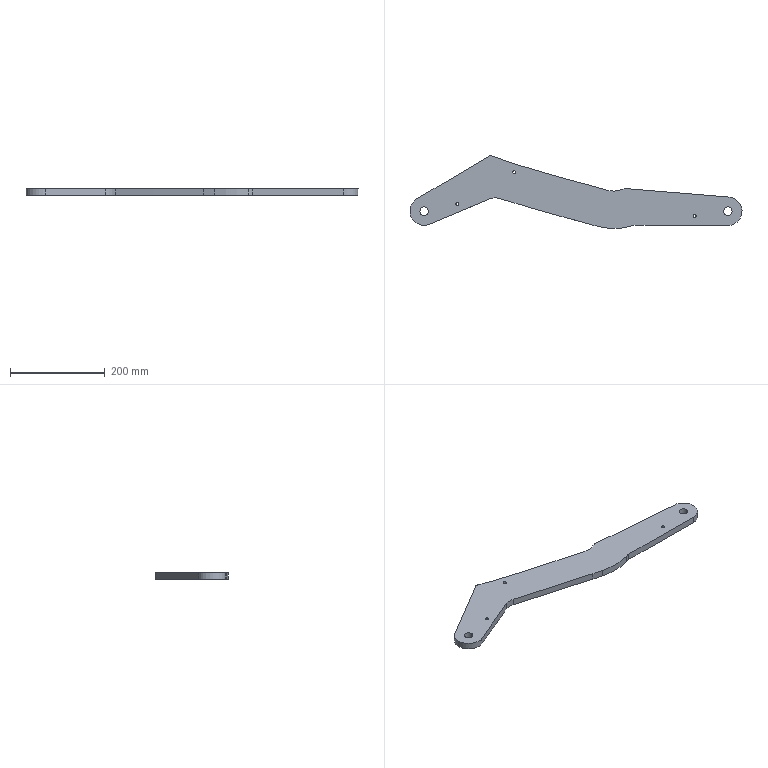NC program | NX | posted with a generic post | part box 700 x 153.975 x 14 mm
Lines 4525 to 6173 of 6173, first 1547 of 1637 lines:
(SPOT_FACING_COPY , TOOL : D12)
N9042 M6
N9044 G54
N9046 G17 G0 G90 X640. Y0. S0 M3
N9048 G43 Z117. H0
N9050 G94 G82 G99 Z17. F250. P200 R23.
N9052 X0.
N9054 G80
N9056 G0 X0. Y0. Z117.
N9058 M5
(ZLEVEL_PROFILE , TOOL : D20R0)
N9060 M6
N9062 G54
N9064 G17 G0 G90 X590.572 Y-39.778 S4500 M3
N9066 G43 Z117. H0
N9068 Z15.
N9070 G94 G1 X639.806 Y-40. Z14.141 F3000.
N9072 X641.356 Y-40.007 Z14.114
N9074 X645.633 Y-39.632 Z14.039
N9076 X649.845 Y-38.8 Z13.964
N9078 X653.944 Y-37.523 Z13.889
N9080 X657.883 Y-35.814 Z13.814
N9082 X661.616 Y-33.692 Z13.739
N9084 X665.1 Y-31.183 Z13.664
N9086 X668.295 Y-28.316 Z13.589
N9088 X671.165 Y-25.122 Z13.514
N9090 X673.677 Y-21.64 Z13.439
N9092 X675.25 Y-18.97 Z13.385
N9094 X677.089 Y-15.059 Z13.31
N9096 X678.497 Y-10.973 Z13.234
N9098 X679.455 Y-6.758 Z13.159
N9100 X679.954 Y-2.465 Z13.083
N9102 X679.987 Y1.857 Z13.008
N9104 X679.554 Y6.157 Z12.932
N9106 X678.659 Y10.385 Z12.857
N9108 X677.314 Y14.493 Z12.781
N9110 X675.534 Y18.431 Z12.706
N9112 X673.34 Y22.155 Z12.631
N9114 X670.757 Y25.62 Z12.555
N9116 X667.816 Y28.787 Z12.48
N9118 X664.55 Y31.618 Z12.404
N9120 X660.998 Y34.08 Z12.329
N9122 X657.202 Y36.146 Z12.253
N9124 X653.205 Y37.789 Z12.178
N9126 X649.053 Y38.993 Z12.102
N9128 X644.797 Y39.742 Z12.027
N9130 X643.252 Y39.868 Z12.
N9132 G2 X639.806 Y-40. R40.
N9134 G1 X448.418 Y-39.138
N9136 G3 X442.249 Y-40.086 R20.
N9138 G2 X365.067 Y-42.198 R139.056
N9140 X207.429 Y1.588 R6700.642
N9142 X163.525 Y14.814 R2452.181
N9144 G1 X156.009 Y17.183
N9146 G3 X142.137 Y16.562 R20.
N9148 G1 X15.549 Y-36.854
N9150 G2 X-20.445 Y34.38 R40.
N9152 G1 Z10.
N9154 G3 X15.549 Y-36.854 R40.
N9156 G1 X142.137 Y16.562
N9158 G2 X156.009 Y17.183 R20.
N9160 G3 X205.106 Y2.266 R2244.387
N9162 X365.066 Y-42.198 R6672.834
N9164 X442.249 Y-40.086 R138.995
N9166 G2 X448.418 Y-39.138 R20.
N9168 G1 X639.806 Y-40.
N9170 G3 X643.252 Y39.868 R40.
N9172 G1 Z8.
N9174 G2 X639.806 Y-40. R40.
N9176 G1 X448.418 Y-39.138
N9178 G3 X442.249 Y-40.086 R20.
N9180 G2 X365.065 Y-42.198 R138.996
N9182 X205.106 Y2.265 R6680.91
N9184 X156.009 Y17.183 R2242.923
N9186 G3 X142.137 Y16.562 R20.
N9188 G1 X15.549 Y-36.854
N9190 G2 X-20.445 Y34.38 R40.
N9192 G1 Z6.
N9194 G3 X15.549 Y-36.854 R40.
N9196 G1 X142.137 Y16.562
N9198 G2 X156.009 Y17.183 R20.
N9200 G3 X205.106 Y2.265 R2241.461
N9202 X364.863 Y-42.146 R6694.497
N9204 X442.249 Y-40.086 R139.003
N9206 G2 X448.418 Y-39.138 R20.
N9208 G1 X639.806 Y-40.
N9210 G3 X643.252 Y39.868 R40.
N9212 G1 Z4.
N9214 G2 X639.806 Y-40. R40.
N9216 G1 X448.418 Y-39.138
N9218 G3 X442.249 Y-40.086 R20.
N9220 G2 X364.863 Y-42.147 R138.995
N9222 X205.106 Y2.264 R6704.295
N9224 X156.009 Y17.183 R2239.999
N9226 G3 X142.137 Y16.562 R20.
N9228 G1 X15.549 Y-36.854
N9230 G2 X-20.445 Y34.38 R40.
N9232 G1 Z2.
N9234 G3 X15.549 Y-36.854 R40.
N9236 G1 X142.137 Y16.562
N9238 G2 X156.009 Y17.183 R20.
N9240 G3 X205.106 Y2.264 R2242.559
N9242 X364.863 Y-42.148 R6672.146
N9244 X442.249 Y-40.086 R138.997
N9246 G2 X448.418 Y-39.138 R20.
N9248 G1 X639.806 Y-40.
N9250 G3 X643.252 Y39.868 R40.
N9252 G1 Z0.
N9254 G2 X639.806 Y-40. R40.
N9256 G1 X448.418 Y-39.138
N9258 G3 X442.249 Y-40.086 R20.
N9260 G2 X364.863 Y-42.148 R138.999
N9262 X205.106 Y2.263 R6621.095
N9264 X156.009 Y17.183 R2197.08
N9266 G3 X142.137 Y16.562 R20.
N9268 G1 X15.549 Y-36.854
N9270 G2 X-20.445 Y34.38 R40.
N9272 G1 Z3.
N9274 G0 Z117.
N9276 M5
(CONTOUR_TEXT , TOOL : D0.1)
N9278 M6
N9280 G54
N9282 G17 G0 G90 X143.989 Y116.042 S2000 M3
N9284 G43 Z117. H0
N9286 Z17.01
N9288 G94 G1 Z14. F1000.
N9290 X140.878 Y26.737
N9292 Z17.01
N9294 G0 Z117.
N9296 X340. Y56.736
N9298 Z17.01
N9300 G1 Z14.
N9302 Y56.686
N9304 Y-25.158
N9306 Z17.01
N9308 G0 Z117.
N9310 X365. Y49.967
N9312 Z17.01
N9314 G1 Z14.
N9316 Y49.902
N9318 Y-31.828
N9320 Y-31.838
N9322 Z17.01
N9324 G0 Z117.
N9326 M5
(SPOT_FACING , TOOL : D18)
N9328 M6
N9330 G54
N9332 G17 G0 G90 X640. Y0. S0 M3
N9334 G43 Z117. H0
N9336 G94 G82 G99 Z14. F250. P200 R20.
N9338 X0.
N9340 G80
N9342 G0 X0. Y0. Z117.
N9344 M5
(SPOT_FACING_1 , TOOL : D6.35)
N9346 M6
N9348 G54
N9350 G17 G0 G90 X570. Y-10. S0 M3
N9352 G43 Z117. H0
N9354 G94 G82 G99 Z14. F250. P200 R20.
N9356 X190. Y82.
N9358 X70. Y15.
N9360 G80
N9362 G0 X70. Y15. Z117.
N9364 M5
(ZLEVEL_PROFILE_COPY_COPY , TOOL : D16R3)
N9366 M6
N9368 G54
N9370 G17 G0 G90 X-407.756 Y50.913 S4500 M3
N9372 G43 Z100. H0
N9374 Z3.015
N9376 G94 G1 Z0.015 F3000.
N9378 G3 X-401.133 Y50.207 R42.151
N9380 G1 Z3.015
N9382 G0 Z100.
N9384 X-387.654 Y52.009
N9386 Z3.015
N9388 G1 Z0.015
N9390 G3 X-383.592 Y53.088 R6599.663
N9392 G1 Z3.015
N9394 G0 Z100.
N9396 X-378.518 Y54.438
N9398 Z3.015
N9400 G1 Z0.015
N9402 G3 X-373.217 Y55.854 R6599.663
N9404 G1 Z3.015
N9406 G0 Z100.
N9408 X-369.755 Y56.781
N9410 Z3.015
N9412 G1 Z0.015
N9414 G3 X-366.871 Y57.555 R6599.663
N9416 G1 Z3.015
N9418 G0 Z100.
N9420 X-358.003 Y59.944
N9422 Z3.015
N9424 G1 Z0.015
N9426 G3 X-352.957 Y61.309 R6599.663
N9428 G1 Z3.015
N9430 G0 Z100.
N9432 X-330.802 Y67.353
N9434 Z3.015
N9436 G1 Z0.015
N9438 G3 X-327.793 Y68.181 R6599.663
N9440 G1 Z3.015
N9442 G0 Z100.
N9444 X-298.143 Y76.415
N9446 Z3.015
N9448 G1 Z0.015
N9450 G3 X-296.135 Y76.978 R6599.663
N9452 G1 Z3.015
N9454 G0 Z100.
N9456 X-290.769 Y78.486
N9458 Z3.015
N9460 G1 Z0.015
N9462 G3 X-288.272 Y79.189 R6599.663
N9464 G1 Z3.015
N9466 G0 Z100.
N9468 X-248.142 Y90.638
N9470 Z3.015
N9472 G1 Z0.015
N9474 G3 X-246.973 Y90.976 R6599.663
N9476 G1 Z3.015
N9478 G0 Z100.
N9480 X-211.221 Y101.494
N9482 Z3.015
N9484 G1 Z0.015
N9486 G3 X-207.58 Y102.599 R2171.481
N9488 G1 Z3.015
N9490 G0 Z100.
N9492 X-153.644 Y120.541
N9494 Z3.015
N9496 G1 Z0.015
N9498 G3 X-150.685 Y121.74 R241.278
N9500 G1 Z3.015
N9502 G0 Z100.
N9504 X-147.619 Y123.03
N9506 Z3.015
N9508 G1 Z0.015
N9510 G3 X-145.285 Y124.045 R241.278
N9512 G2 X-141.102 Y125.139 R12.975
N9514 G1 Z3.015
N9516 G0 Z100.
N9518 X-415.341 Y53.085
N9520 Z3.015
N9522 G1 Z0.015
N9524 G3 X-411.202 Y51.709 R42.151
N9526 G1 Z3.015
N9528 G0 Z100.
N9530 X-125.772 Y118.879
N9532 Z2.866
N9534 G1 X19.35 Y32.635 Z-0.081
N9536 X21.902 Y31.119 Z-0.133
N9538 X21.939 Y31.096 Z-0.134
N9540 X21.976 Y31.074
N9542 X21.902 Y31.119
N9544 X19.35 Y32.635
N9546 X-133.408 Y123.417
N9548 G3 X-145.285 Y124.046 R12.983
N9550 G2 X-161.394 Y117.61 R244.177
N9552 X-192.374 Y107.278 R743.347
N9554 X-243.617 Y91.937 R2595.945
N9556 X-389.036 Y51.644 R6726.527
N9558 X-418.12 Y54.295 R42.063
N9560 G3 X-424.947 Y55.612 R13.128
N9562 G1 X-643.044 Y37.818
N9564 X-645.25 Y37.626
N9566 Z-0.284
N9568 X-643.044 Y37.818
N9570 X-424.947 Y55.612
N9572 G2 X-418.12 Y54.295 R13.112
N9574 G3 X-389.036 Y51.645 R42.063
N9576 X-243.617 Y91.938 R6726.001
N9578 X-192.374 Y107.278 R2596.179
N9580 X-161.396 Y117.61 R743.332
N9582 X-145.285 Y124.047 R244.134
N9584 G2 X-133.408 Y123.417 R12.974
N9586 G1 X19.35 Y32.635
N9588 X21.902 Y31.119
N9590 X21.976 Y31.074
N9592 Z-0.433
N9594 X21.902 Y31.119
N9596 X19.35 Y32.635
N9598 X-133.408 Y123.417
N9600 G3 X-145.285 Y124.048 R12.971
N9602 G2 X-161.398 Y117.61 R244.08
N9604 X-192.374 Y107.279 R743.308
N9606 X-243.617 Y91.938 R2596.414
N9608 X-389.036 Y51.645 R6725.354
N9610 X-418.12 Y54.296 R42.063
N9612 G3 X-424.947 Y55.612 R13.096
N9614 G1 X-643.044 Y37.818
N9616 X-645.25 Y37.626
N9618 Z-0.582
N9620 X-643.044 Y37.818
N9622 X-424.947 Y55.612
N9624 G2 X-418.12 Y54.297 R13.085
N9626 G3 X-389.036 Y51.646 R42.063
N9628 X-243.617 Y91.939 R6724.841
N9630 X-192.374 Y107.28 R2596.46
N9632 X-161.4 Y117.61 R743.27
N9634 X-145.285 Y124.049 R244.026
N9636 G2 X-133.408 Y123.417 R12.969
N9638 G1 X19.35 Y32.635
N9640 X21.902 Y31.119
N9642 X21.976 Y31.074
N9644 Z-0.731
N9646 X21.902 Y31.119
N9648 X19.35 Y32.635
N9650 X-133.408 Y123.417
N9652 G3 X-145.285 Y124.05 R12.969
N9654 G2 X-161.402 Y117.61 R243.973
N9656 X-192.374 Y107.28 R743.229
N9658 X-243.617 Y91.94 R2596.058
N9660 X-389.036 Y51.647 R6724.335
N9662 X-418.12 Y54.298 R42.063
N9664 G3 X-424.947 Y55.612 R13.081
N9666 G1 X-643.044 Y37.818
N9668 X-645.25 Y37.626
N9670 Z-0.881
N9672 X-643.044 Y37.818
N9674 X-424.947 Y55.612
N9676 G2 X-418.12 Y54.299 R13.079
N9678 G3 X-389.036 Y51.648 R42.062
N9680 X-243.617 Y91.94 R6723.829
N9682 X-192.374 Y107.281 R2595.627
N9684 X-161.404 Y117.61 R743.186
N9686 X-145.285 Y124.05 R243.919
N9688 G2 X-133.408 Y123.417 R12.969
N9690 G1 X19.35 Y32.635
N9692 X21.902 Y31.119
N9694 X21.976 Y31.074
N9696 Z-1.03
N9698 X21.902 Y31.119
N9700 X19.35 Y32.635
N9702 X-133.408 Y123.417
N9704 G3 X-145.285 Y124.051 R12.968
N9706 G2 X-161.406 Y117.61 R243.88
N9708 X-192.374 Y107.282 R743.005
N9710 X-243.617 Y91.941 R2595.195
N9712 X-389.036 Y51.648 R6723.968
N9714 X-418.12 Y54.299 R42.063
N9716 G3 X-424.947 Y55.612 R13.077
N9718 G1 X-643.044 Y37.818
N9720 X-645.25 Y37.626
N9722 X-645.251 Y37.638 Z-1.179
N9724 X-643.044 Y37.818
N9726 X-424.947 Y55.612
N9728 G2 X-418.12 Y54.3 R13.075
N9730 G3 X-389.036 Y51.649 R42.063
N9732 X-243.617 Y91.942 R6724.339
N9734 X-192.374 Y107.282 R2594.764
N9736 X-161.408 Y117.61 R743.099
N9738 X-145.285 Y124.052 R243.869
N9740 G2 X-133.408 Y123.417 R12.968
N9742 G1 X19.35 Y32.635
N9744 X21.902 Y31.119
N9746 X21.976 Y31.074
N9748 Z-1.328
N9750 X19.35 Y32.635
N9752 X-133.408 Y123.417
N9754 G3 X-145.285 Y124.053 R12.968
N9756 G2 X-161.409 Y117.61 R243.819
N9758 X-192.374 Y107.283 R743.193
N9760 X-243.617 Y91.942 R2594.333
N9762 X-389.036 Y51.65 R6724.711
N9764 X-418.12 Y54.301 R42.062
N9766 G3 X-424.947 Y55.612 R13.073
N9768 G1 X-643.044 Y37.818
N9770 X-645.251 Y37.638
N9772 Z-1.478
N9774 X-643.044 Y37.818
N9776 X-424.947 Y55.612
N9778 G2 X-418.12 Y54.302 R13.071
N9780 G3 X-389.036 Y51.651 R42.061
N9782 X-243.617 Y91.943 R6725.083
N9784 X-192.374 Y107.284 R2593.902
N9786 X-161.411 Y117.61 R743.288
N9788 X-145.285 Y124.054 R243.688
N9790 G2 X-133.408 Y123.417 R12.968
N9792 G1 X19.35 Y32.635
N9794 X21.902 Y31.119
N9796 X21.976 Y31.074
N9798 Z-1.627
N9800 X21.902 Y31.119
N9802 X19.35 Y32.635
N9804 X-133.408 Y123.417
N9806 G3 X-145.285 Y124.055 R12.968
N9808 G2 X-161.413 Y117.61 R243.517
N9810 X-192.374 Y107.284 R743.382
N9812 X-243.617 Y91.944 R2593.471
N9814 X-389.036 Y51.651 R6725.454
N9816 X-418.12 Y54.303 R42.06
N9818 G3 X-424.947 Y55.612 R13.069
N9820 G1 X-643.044 Y37.818
N9822 X-645.25 Y37.626
N9824 Z-1.776
N9826 X-643.044 Y37.818
N9828 X-424.947 Y55.612
N9830 G2 X-418.12 Y54.303 R13.068
N9832 G3 X-389.036 Y51.652 R42.059
N9834 X-243.617 Y91.944 R6725.826
N9836 X-193.759 Y106.853 R2626.625
N9838 X-163.29 Y116.934 R784.546
N9840 X-145.285 Y124.056 R254.256
N9842 G2 X-133.408 Y123.417 R12.97
N9844 G1 X19.35 Y32.635
N9846 X21.976 Y31.074
N9848 Z-1.925
N9850 X19.35 Y32.635
N9852 X-133.408 Y123.417
N9854 G3 X-145.285 Y124.057 R12.971
N9856 G2 X-163.29 Y116.935 R253.869
N9858 X-193.759 Y106.853 R784.382
N9860 X-243.617 Y91.945 R2625.972
N9862 X-389.036 Y51.653 R6726.197
N9864 X-418.12 Y54.304 R42.058
N9866 G3 X-424.947 Y55.612 R13.067
N9868 G1 X-643.044 Y37.818
N9870 X-645.25 Y37.626
N9872 Z-2.075
N9874 X-643.044 Y37.818
N9876 X-424.947 Y55.612
N9878 G2 X-418.12 Y54.305 R13.066
N9880 G3 X-389.036 Y51.653 R42.057
N9882 X-243.617 Y91.945 R6727.425
N9884 X-192.374 Y107.286 R2594.029
N9886 X-161.418 Y117.61 R742.762
N9888 X-145.285 Y124.058 R242.584
N9890 G2 X-133.408 Y123.417 R12.972
N9892 G1 X19.35 Y32.635
N9894 X21.976 Y31.074
N9896 Z-2.224
N9898 X19.35 Y32.635
N9900 X-133.408 Y123.417
N9902 G3 X-145.285 Y124.059 R12.974
N9904 G2 X-161.42 Y117.61 R242.183
N9906 X-192.374 Y107.286 R741.914
N9908 X-243.617 Y91.946 R2595.715
N9910 X-389.036 Y51.654 R6732.513
N9912 X-418.12 Y54.306 R42.055
N9914 G3 X-424.947 Y55.612 R13.067
N9916 G1 X-643.044 Y37.818
N9918 X-645.25 Y37.626
N9920 Z-2.373
N9922 X-643.044 Y37.818
N9924 X-424.947 Y55.612
N9926 G2 X-418.12 Y54.306 R13.072
N9928 G3 X-389.036 Y51.654 R42.054
N9930 X-232.193 Y95.277 R6557.333
N9932 X-186.834 Y109.038 R2105.117
N9934 X-161.422 Y117.61 R671.478
N9936 X-145.285 Y124.06 R241.607
N9938 G2 X-133.408 Y123.417 R12.976
N9940 G1 X19.35 Y32.635
N9942 X21.976 Y31.074
N9944 Z-2.522
N9946 X19.35 Y32.635
N9948 X-133.408 Y123.417
N9950 G3 X-145.285 Y124.061 R12.976
N9952 G2 X-161.423 Y117.61 R241.158
N9954 X-186.834 Y109.038 R670.893
N9956 X-233.922 Y94.773 R2161.711
N9958 X-389.036 Y51.655 R6568.584
N9960 X-418.12 Y54.307 R42.052
N9962 G3 X-424.947 Y55.612 R13.079
N9964 G1 X-643.044 Y37.818
N9966 X-645.25 Y37.626
N9968 Z-2.672
N9970 X-643.044 Y37.818
N9972 X-424.947 Y55.612
N9974 G2 X-418.12 Y54.308 R13.085
N9976 G3 X-389.036 Y51.655 R42.05
N9978 X-235.307 Y94.369 R6591.52
N9980 X-189.604 Y108.163 R2253.663
N9982 X-161.425 Y117.61 R696.975
N9984 X-145.285 Y124.062 R240.518
N9986 G2 X-133.408 Y123.417 R12.977
N9988 G1 X19.35 Y32.635
N9990 X21.976 Y31.074
N9992 Z-2.821
N9994 X19.35 Y32.635
N9996 X-133.408 Y123.417
N9998 G3 X-145.285 Y124.063 R12.978
N10000 G2 X-161.427 Y117.61 R243.838
N10002 X-189.604 Y108.163 R697.021
N10004 X-232.583 Y95.164 R2231.213
N10006 X-389.036 Y51.656 R6582.428
N10008 X-418.12 Y54.309 R42.048
N10010 G3 X-424.947 Y55.612 R13.091
N10012 G1 X-643.044 Y37.818
N10014 X-645.25 Y37.626
N10016 Z-2.97
N10018 X-643.044 Y37.818
N10020 X-424.947 Y55.612
N10022 G2 X-418.12 Y54.31 R13.097
N10024 G3 X-389.036 Y51.656 R42.046
N10026 X-235.307 Y94.37 R6605.781
N10028 X-186.834 Y109.04 R2185.124
N10030 X-161.429 Y117.61 R678.962
N10032 X-145.285 Y124.064 R243.704
N10034 G2 X-133.408 Y123.417 R12.98
N10036 G1 X19.35 Y32.635
N10038 X21.976 Y31.074
N10040 Z-3.119
N10042 X19.383 Y32.615
N10044 X-133.408 Y123.417
N10046 G3 X-145.285 Y124.065 R12.956
N10048 G2 X-160.135 Y118.088 R230.666
N10050 X-186.834 Y109.042 R650.105
N10052 X-232.454 Y95.204 R2166.728
N10054 X-388.833 Y51.712 R6643.891
N10056 X-418.12 Y54.311 R42.064
N10058 G3 X-424.925 Y55.614 R12.998
N10060 G1 X-643.085 Y37.814
N10062 X-645.25 Y37.626
N10064 Z-3.269
N10066 X-643.085 Y37.814
N10068 X-424.923 Y55.614
N10070 G2 X-418.12 Y54.311 R13.
N10072 G3 X-388.836 Y51.712 R42.063
N10074 X-232.454 Y95.205 R6643.863
N10076 X-186.834 Y109.043 R2167.21
N10078 X-160.135 Y118.088 R649.315
N10080 X-145.285 Y124.066 R230.896
N10082 G2 X-133.408 Y123.417 R12.956
N10084 G1 X19.383 Y32.615
N10086 X21.976 Y31.074
N10088 Z-3.418
N10090 X19.383 Y32.615
N10092 X-133.408 Y123.417
N10094 G3 X-145.285 Y124.067 R12.956
N10096 G2 X-160.135 Y118.089 R230.903
N10098 X-186.834 Y109.043 R646.14
N10100 X-232.455 Y95.206 R2167.693
N10102 X-388.839 Y51.712 R6643.82
N10104 X-418.12 Y54.312 R42.062
N10106 G3 X-424.922 Y55.614 R13.002
N10108 G1 X-643.085 Y37.814
N10110 X-645.25 Y37.626
N10112 Z-3.567
N10114 X-643.085 Y37.814
N10116 X-424.92 Y55.614
N10118 G2 X-418.12 Y54.313 R13.004
N10120 G3 X-388.842 Y51.712 R42.061
N10122 X-232.455 Y95.206 R6643.759
N10124 X-186.834 Y109.044 R2168.176
N10126 X-160.136 Y118.09 R659.938
N10128 X-145.285 Y124.068 R230.911
N10130 G2 X-133.408 Y123.417 R12.957
N10132 G1 X19.383 Y32.615
N10134 X21.976 Y31.074
N10136 Z-3.716
N10138 X19.383 Y32.615
N10140 X-133.408 Y123.417
N10142 G3 X-145.285 Y124.069 R12.957
N10144 G2 X-160.136 Y118.09 R230.918
N10146 X-186.834 Y109.044 R659.332
N10148 X-232.455 Y95.207 R2168.659
N10150 X-389.036 Y51.662 R6578.665
N10152 X-418.12 Y54.314 R42.043
N10154 G3 X-424.919 Y55.614 R13.006
N10156 G1 X-643.085 Y37.814
N10158 X-645.25 Y37.626
N10160 Z-3.866
N10162 X-643.085 Y37.814
N10164 X-424.917 Y55.614
N10166 G2 X-418.12 Y54.315 R13.009
N10168 G3 X-389.036 Y51.663 R42.042
N10170 X-232.455 Y95.208 R6578.599
N10172 X-186.834 Y109.045 R2169.142
N10174 X-160.136 Y118.091 R661.011
N10176 X-145.285 Y124.069 R230.926
N10178 G2 X-133.408 Y123.417 R12.957
N10180 G1 X19.383 Y32.615
N10182 X21.976 Y31.074
N10184 Z-4.015
N10186 X19.383 Y32.615
N10188 X-133.408 Y123.417
N10190 G3 X-145.285 Y124.07 R12.957
N10192 G2 X-160.136 Y118.092 R230.933
N10194 X-186.834 Y109.046 R662.697
N10196 X-232.455 Y95.208 R2169.685
N10198 X-389.036 Y51.663 R6579.068
N10200 X-418.12 Y54.316 R42.042
N10202 G3 X-424.916 Y55.614 R13.011
N10204 G1 X-643.085 Y37.814
N10206 X-645.25 Y37.626
N10208 Z-4.164
N10210 X-643.085 Y37.814
N10212 X-424.914 Y55.614
N10214 G2 X-418.12 Y54.316 R13.013
N10216 G3 X-389.036 Y51.664 R42.041
N10218 X-232.456 Y95.209 R6579.537
N10220 X-186.834 Y109.046 R2171.653
N10222 X-160.137 Y118.092 R647.182
N10224 X-145.285 Y124.071 R230.94
N10226 G2 X-133.408 Y123.417 R12.958
N10228 G1 X19.383 Y32.615
N10230 X21.976 Y31.074
N10232 Z-4.313
N10234 X19.383 Y32.615
N10236 X-133.408 Y123.417
N10238 G3 X-145.285 Y124.072 R12.958
N10240 G2 X-160.137 Y118.093 R237.294
N10242 X-186.834 Y109.047 R647.939
N10244 X-232.196 Y95.287 R2151.551
N10246 X-389.036 Y51.665 R6615.728
N10248 X-418.12 Y54.317 R42.04
N10250 G3 X-424.913 Y55.615 R13.015
N10252 G1 X-643.085 Y37.814
N10254 X-645.25 Y37.626
N10256 Z-4.463
N10258 X-643.085 Y37.814
N10260 X-424.911 Y55.615
N10262 G2 X-418.12 Y54.318 R13.017
N10264 G3 X-389.036 Y51.666 R42.04
N10266 X-232.456 Y95.21 R6579.217
N10268 X-186.834 Y109.048 R2169.86
N10270 X-160.137 Y118.094 R648.556
N10272 X-145.285 Y124.073 R237.332
N10274 G2 X-133.408 Y123.417 R12.958
N10276 G1 X19.383 Y32.615
N10278 X21.976 Y31.074
N10280 Z-4.612
N10282 X19.383 Y32.615
N10284 X-133.408 Y123.417
N10286 G3 X-145.285 Y124.074 R12.958
N10288 G2 X-160.137 Y118.094 R237.469
N10290 X-186.834 Y109.048 R648.403
N10292 X-232.456 Y95.211 R2169.799
N10294 X-389.036 Y51.667 R6579.826
N10296 X-418.12 Y54.319 R42.039
N10298 G3 X-424.91 Y55.615 R13.019
N10300 G1 X-643.085 Y37.814
N10302 X-645.25 Y37.626
N10304 Z-4.761
N10306 X-643.085 Y37.814
N10308 X-424.908 Y55.615
N10310 G2 X-418.12 Y54.32 R13.022
N10312 G3 X-389.036 Y51.667 R42.039
N10314 X-232.456 Y95.211 R6581.414
N10316 X-186.834 Y109.049 R2169.738
N10318 X-160.138 Y118.095 R648.249
N10320 X-145.285 Y124.075 R231.343
N10322 G2 X-133.408 Y123.417 R12.959
N10324 G1 X19.383 Y32.615
N10326 X21.976 Y31.074
N10328 Z-4.91
N10330 X19.383 Y32.615
N10332 X-133.408 Y123.417
N10334 G3 X-145.285 Y124.075 R12.959
N10336 G2 X-160.138 Y118.095 R231.329
N10338 X-186.834 Y109.05 R648.058
N10340 X-232.456 Y95.212 R2169.677
N10342 X-389.036 Y51.668 R6581.883
N10344 X-418.12 Y54.321 R42.038
N10346 G3 X-424.907 Y55.615 R13.024
N10348 G1 X-643.085 Y37.814
N10350 X-645.25 Y37.626
N10352 Z-5.06
N10354 X-643.085 Y37.814
N10356 X-424.905 Y55.615
N10358 G2 X-418.12 Y54.321 R13.026
N10360 G3 X-389.036 Y51.669 R42.037
N10362 X-232.457 Y95.212 R6582.352
N10364 X-186.834 Y109.05 R2169.616
N10366 X-160.138 Y118.096 R648.698
N10368 X-145.285 Y124.076 R231.313
N10370 G2 X-133.408 Y123.417 R12.959
N10372 G1 X19.383 Y32.615
N10374 X21.976 Y31.074
N10376 Z-5.209
N10378 X19.383 Y32.615
N10380 X-133.408 Y123.417
N10382 G3 X-145.285 Y124.077 R12.96
N10384 G2 X-160.138 Y118.097 R231.297
N10386 X-186.834 Y109.051 R649.34
N10388 X-232.457 Y95.213 R2169.555
N10390 X-389.036 Y51.67 R6582.822
N10392 X-418.12 Y54.322 R42.037
N10394 G3 X-424.904 Y55.615 R13.
N10396 G1 X-643.085 Y37.814
N10398 X-645.25 Y37.626
N10400 Z-5.358
N10402 X-643.085 Y37.814
N10404 X-424.902 Y55.615
N10406 G2 X-418.12 Y54.323 R13.002
N10408 G3 X-389.036 Y51.67 R42.036
N10410 X-232.457 Y95.214 R6649.547
N10412 X-186.834 Y109.052 R2169.494
N10414 X-160.139 Y118.097 R649.984
N10416 X-145.285 Y124.078 R231.282
N10418 G2 X-133.408 Y123.417 R12.96
N10420 G1 X19.383 Y32.615
N10422 X21.976 Y31.074
N10424 Z-5.507
N10426 X19.383 Y32.615
N10428 X-133.408 Y123.417
N10430 G3 X-145.285 Y124.079 R12.96
N10432 G2 X-160.139 Y118.098 R231.267
N10434 X-186.834 Y109.052 R650.629
N10436 X-232.457 Y95.214 R2169.433
N10438 X-389.036 Y51.671 R6649.11
N10440 X-418.12 Y54.324 R42.035
N10442 G3 X-424.901 Y55.616 R13.005
N10444 G1 X-643.085 Y37.814
N10446 X-645.25 Y37.626
N10448 Z-5.657
N10450 X-643.085 Y37.814
N10452 X-424.899 Y55.616
N10454 G2 X-418.12 Y54.325 R13.007
N10456 G3 X-389.036 Y51.672 R42.035
N10458 X-232.457 Y95.215 R6648.673
N10460 X-186.834 Y109.053 R2169.372
N10462 X-160.139 Y118.099 R651.277
N10464 X-145.285 Y124.08 R231.253
N10466 G2 X-133.408 Y123.417 R12.96
N10468 G1 X19.383 Y32.615
N10470 X21.976 Y31.074
N10472 Z-5.806
N10474 X19.383 Y32.615
N10476 X-133.408 Y123.417
N10478 G3 X-145.285 Y124.081 R12.961
N10480 G2 X-160.139 Y118.099 R231.238
N10482 X-186.834 Y109.054 R651.926
N10484 X-232.457 Y95.215 R2169.311
N10486 X-389.036 Y51.673 R6648.236
N10488 X-418.12 Y54.326 R42.034
N10490 G3 X-424.898 Y55.616 R13.009
N10492 G1 X-643.085 Y37.814
N10494 X-645.25 Y37.626
N10496 Z-5.955
N10498 X-643.085 Y37.814
N10500 X-424.896 Y55.616
N10502 G2 X-418.12 Y54.326 R13.011
N10504 G3 X-389.036 Y51.673 R42.033
N10506 X-232.458 Y95.216 R6647.799
N10508 X-186.834 Y109.054 R2169.25
N10510 X-160.14 Y118.1 R652.577
N10512 X-145.285 Y124.082 R231.223
N10514 G2 X-133.408 Y123.417 R12.961
N10516 G1 X19.383 Y32.615
N10518 X21.976 Y31.074
N10520 Z-6.104
N10522 X19.383 Y32.615
N10524 X-133.408 Y123.417
N10526 G3 X-145.285 Y124.082 R12.962
N10528 G2 X-160.14 Y118.101 R231.208
N10530 X-186.834 Y109.055 R653.23
N10532 X-232.458 Y95.217 R2169.189
N10534 X-389.036 Y51.674 R6647.362
N10536 X-418.12 Y54.327 R42.033
N10538 G3 X-424.895 Y55.616 R13.013
N10540 G1 X-643.085 Y37.814
N10542 X-645.25 Y37.626
N10544 Z-6.254
N10546 X-643.085 Y37.814
N10548 X-424.893 Y55.616
N10550 G2 X-418.12 Y54.328 R13.015
N10552 G3 X-389.036 Y51.675 R42.032
N10554 X-232.458 Y95.217 R6646.926
N10556 X-186.834 Y109.056 R2164.138
N10558 X-160.14 Y118.101 R652.975
N10560 X-145.285 Y124.083 R231.193
N10562 G2 X-133.408 Y123.417 R12.963
N10564 G1 X19.383 Y32.615
N10566 X21.976 Y31.074
N10568 Z-6.403
N10570 X19.383 Y32.615
N10572 X-133.408 Y123.417
N10574 G3 X-145.285 Y124.084 R12.963
N10576 G2 X-160.14 Y118.102 R231.178
N10578 X-186.834 Y109.056 R652.668
N10580 X-232.458 Y95.218 R2164.759
N10582 X-389.036 Y51.676 R6640.274
N10584 X-418.12 Y54.329 R42.031
N10586 G3 X-424.892 Y55.616 R13.018
N10588 G1 X-643.085 Y37.814
N10590 X-645.25 Y37.626
N10592 Z-6.552
N10594 X-643.085 Y37.814
N10596 X-424.89 Y55.616
N10598 G2 X-418.12 Y54.33 R13.02
N10600 G3 X-389.036 Y51.676 R42.031
N10602 X-232.458 Y95.219 R6640.262
N10604 X-186.834 Y109.057 R2165.381
N10606 X-160.14 Y118.103 R652.361
N10608 X-145.285 Y124.085 R231.163
N10610 G2 X-133.408 Y123.417 R12.964
N10612 G1 X19.383 Y32.615
N10614 X21.976 Y31.074
N10616 Z-6.701
N10618 X19.383 Y32.615
N10620 X-133.408 Y123.417
N10622 G3 X-145.285 Y124.086 R12.965
N10624 G2 X-160.141 Y118.103 R231.148
N10626 X-186.834 Y109.057 R652.054
N10628 X-232.459 Y95.219 R2163.102
N10630 X-389.036 Y51.677 R6640.25
N10632 X-418.12 Y54.331 R42.03
N10634 G3 X-424.889 Y55.617 R13.022
N10636 G1 X-643.085 Y37.814
N10638 X-645.25 Y37.626
N10640 Z-6.851
N10642 X-643.085 Y37.814
N10644 X-424.887 Y55.617
N10646 G2 X-418.12 Y54.331 R13.024
N10648 G3 X-389.036 Y51.678 R42.03
N10650 X-232.459 Y95.22 R6640.238
N10652 X-186.834 Y109.058 R2163.96
N10654 X-160.141 Y118.104 R651.747
N10656 X-145.285 Y124.087 R231.133
N10658 G2 X-133.408 Y123.417 R12.966
N10660 G1 X19.383 Y32.615
N10662 X21.976 Y31.074
N10664 Z-7.
N10666 X19.383 Y32.615
N10668 X-133.408 Y123.417
N10670 G3 X-145.285 Y124.088 R12.967
N10672 G2 X-160.141 Y118.104 R231.09
N10674 X-186.834 Y109.059 R651.441
N10676 X-232.459 Y95.22 R2164.819
N10678 X-389.036 Y51.679 R6640.226
N10680 X-418.12 Y54.332 R42.029
N10682 G3 X-424.886 Y55.617 R13.026
N10684 G1 X-643.085 Y37.814
N10686 X-645.25 Y37.626
N10688 Z-7.149
N10690 X-643.085 Y37.814
N10692 X-424.884 Y55.617
N10694 G2 X-418.12 Y54.333 R13.028
N10696 G3 X-389.036 Y51.679 R42.028
N10698 X-232.459 Y95.221 R6640.213
N10700 X-186.834 Y109.059 R2165.679
N10702 X-160.141 Y118.105 R651.134
N10704 X-145.285 Y124.088 R231.032
N10706 G2 X-133.408 Y123.417 R12.968
N10708 G1 X19.383 Y32.615
N10710 X21.976 Y31.074
N10712 Z-7.299
N10714 X19.383 Y32.615
N10716 X-133.408 Y123.417
N10718 G3 X-145.285 Y124.089 R12.968
N10720 G2 X-160.142 Y118.106 R230.973
N10722 X-186.834 Y109.06 R650.828
N10724 X-232.459 Y95.222 R2166.54
N10726 X-389.036 Y51.68 R6640.201
N10728 X-418.12 Y54.334 R42.028
N10730 G3 X-424.883 Y55.617 R13.031
N10732 G1 X-643.085 Y37.814
N10734 X-645.25 Y37.626
N10736 Z-7.448
N10738 X-643.085 Y37.814
N10740 X-424.881 Y55.617
N10742 G2 X-418.12 Y54.335 R13.033
N10744 G3 X-389.036 Y51.681 R42.027
N10746 X-232.459 Y95.222 R6640.188
N10748 X-186.834 Y109.061 R2169.121
N10750 X-160.142 Y118.106 R650.522
N10752 X-145.285 Y124.09 R230.914
N10754 G2 X-133.408 Y123.417 R12.969
N10756 G1 X19.383 Y32.615
N10758 X21.976 Y31.074
N10760 Z-7.597
N10762 X19.383 Y32.615
N10764 X-133.408 Y123.417
N10766 G3 X-145.285 Y124.091 R12.97
N10768 G2 X-160.142 Y118.107 R230.855
N10770 X-186.834 Y109.061 R650.216
N10772 X-232.46 Y95.223 R2169.745
N10774 X-389.036 Y51.682 R6640.176
N10776 X-418.12 Y54.336 R42.026
N10778 G3 X-424.88 Y55.617 R13.035
N10780 G1 X-643.085 Y37.814
N10782 X-645.25 Y37.626
N10784 Z-7.746
N10786 X-643.085 Y37.814
N10788 X-424.878 Y55.617
N10790 G2 X-418.12 Y54.336 R13.037
N10792 G3 X-389.036 Y51.683 R42.026
N10794 X-232.46 Y95.223 R6640.163
N10796 X-186.834 Y109.062 R2170.37
N10798 X-160.142 Y118.108 R649.911
N10800 X-145.285 Y124.092 R230.796
N10802 G2 X-133.408 Y123.417 R12.971
N10804 G1 X19.383 Y32.615
N10806 X21.976 Y31.074
N10808 Z-7.896
N10810 X19.383 Y32.615
N10812 X-133.408 Y123.417
N10814 G3 X-145.285 Y124.093 R12.972
N10816 G2 X-160.143 Y118.108 R230.737
N10818 X-186.834 Y109.063 R649.606
N10820 X-232.46 Y95.224 R2170.995
N10822 X-389.036 Y51.683 R6640.15
N10824 X-418.12 Y54.337 R42.025
N10826 G3 X-424.877 Y55.617 R13.038
N10828 G1 X-643.085 Y37.814
N10830 X-645.25 Y37.626
N10832 Z-8.045
N10834 X-643.085 Y37.814
N10836 X-424.875 Y55.618
N10838 G2 X-418.12 Y54.338 R13.04
N10840 G3 X-389.036 Y51.684 R42.024
N10842 X-232.46 Y95.225 R6640.137
N10844 X-186.834 Y109.063 R2171.621
N10846 X-160.143 Y118.109 R649.3
N10848 X-145.285 Y124.094 R230.679
N10850 G2 X-133.408 Y123.417 R12.973
N10852 G1 X19.383 Y32.615
N10854 X21.976 Y31.074
N10856 Z-8.194
N10858 X19.383 Y32.615
N10860 X-133.408 Y123.417
N10862 G3 X-145.285 Y124.095 R12.973
N10864 G2 X-160.143 Y118.11 R230.62
N10866 X-186.834 Y109.064 R648.995
N10868 X-232.46 Y95.225 R2172.247
N10870 X-389.036 Y51.685 R6640.124
N10872 X-418.12 Y54.339 R42.023
N10874 G3 X-424.874 Y55.618 R13.041
N10876 G1 X-643.085 Y37.814
N10878 X-645.25 Y37.626
N10880 Z-8.343
N10882 X-643.085 Y37.814
N10884 X-424.872 Y55.618
N10886 G2 X-418.12 Y54.34 R13.043
N10888 G3 X-389.036 Y51.686 R42.023
N10890 X-232.461 Y95.226 R6640.111
N10892 X-186.834 Y109.065 R2172.873
N10894 X-160.143 Y118.11 R648.691
N10896 X-145.285 Y124.095 R230.284
N10898 G2 X-133.408 Y123.417 R12.974
N10900 G1 X19.383 Y32.615
N10902 X21.976 Y31.074
N10904 Z-8.493
N10906 X19.383 Y32.615
N10908 X-133.408 Y123.417
N10910 G3 X-145.285 Y124.096 R12.975
N10912 G2 X-160.144 Y118.111 R230.247
N10914 X-186.834 Y109.065 R648.386
N10916 X-232.461 Y95.226 R2173.5
N10918 X-389.036 Y51.686 R6640.098
N10920 X-418.12 Y54.341 R42.022
N10922 G3 X-424.871 Y55.618 R13.044
N10924 G1 X-643.085 Y37.814
N10926 X-645.25 Y37.626
N10928 Z-8.642
N10930 X-643.085 Y37.814
N10932 X-424.869 Y55.618
N10934 G2 X-418.12 Y54.341 R13.045
N10936 G3 X-389.036 Y51.687 R42.021
N10938 X-232.461 Y95.227 R6639.946
N10940 X-186.834 Y109.066 R2174.324
N10942 X-160.144 Y118.112 R648.081
N10944 X-145.285 Y124.097 R230.211
N10946 G2 X-133.408 Y123.417 R12.976
N10948 G1 X19.383 Y32.615
N10950 X21.976 Y31.074
N10952 Z-8.791
N10954 X19.383 Y32.615
N10956 X-133.408 Y123.417
N10958 G3 X-145.285 Y124.098 R12.977
N10960 G2 X-160.144 Y118.112 R230.174
N10962 X-186.834 Y109.067 R647.777
N10964 X-232.461 Y95.228 R2175.194
N10966 X-389.036 Y51.688 R6639.511
N10968 X-418.12 Y54.342 R42.02
N10970 G3 X-424.868 Y55.618 R13.047
N10972 G1 X-643.085 Y37.814
N10974 X-645.25 Y37.626
N10976 Z-8.94
N10978 X-643.085 Y37.814
N10980 X-424.866 Y55.618
N10982 G2 X-418.12 Y54.343 R13.048
N10984 G3 X-389.036 Y51.689 R42.019
N10986 X-232.461 Y95.228 R6639.075
N10988 X-186.834 Y109.067 R2176.064
N10990 X-160.144 Y118.113 R660.973
N10992 X-145.285 Y124.099 R230.137
N10994 G2 X-133.408 Y123.417 R12.978
N10996 G1 X19.383 Y32.615
N10998 X21.976 Y31.074
N11000 Z-9.09
N11002 X19.383 Y32.615
N11004 X-133.408 Y123.417
N11006 G3 X-145.285 Y124.1 R12.978
N11008 G2 X-160.145 Y118.113 R230.1
N11010 X-186.834 Y109.068 R660.757
N11012 X-232.461 Y95.229 R2176.934
N11014 X-388.95 Y51.712 R6640.112
N11016 X-418.12 Y54.344 R42.026
N11018 G3 X-424.865 Y55.618 R13.05
N11020 G1 X-643.085 Y37.814
N11022 X-645.25 Y37.626
N11024 Z-9.239
N11026 X-643.085 Y37.814
N11028 X-424.863 Y55.619
N11030 G2 X-418.12 Y54.345 R13.051
N11032 G3 X-388.953 Y51.712 R42.025
N11034 X-232.462 Y95.23 R6639.625
N11036 X-186.834 Y109.069 R2177.806
N11038 X-160.145 Y118.114 R660.541
N11040 X-145.285 Y124.101 R230.063
N11042 G2 X-133.408 Y123.417 R12.979
N11044 G1 X19.383 Y32.615
N11046 X21.976 Y31.074
N11048 Z-9.388
N11050 X19.383 Y32.615
N11052 X-133.408 Y123.417
N11054 G3 X-145.285 Y124.101 R12.98
N11056 G2 X-160.145 Y118.115 R230.026
N11058 X-186.834 Y109.069 R660.326
N11060 X-232.462 Y95.23 R2178.679
N11062 X-388.956 Y51.712 R6639.139
N11064 X-418.12 Y54.346 R42.024
N11066 G3 X-424.862 Y55.619 R13.053
N11068 G1 X-643.085 Y37.814
N11070 X-645.25 Y37.626
N11072 Z-9.537
N11074 X-643.085 Y37.814
N11076 X-424.86 Y55.619
N11078 G2 X-418.12 Y54.346 R13.054
N11080 G3 X-388.959 Y51.712 R42.023
N11082 X-232.462 Y95.231 R6638.652
N11084 X-186.834 Y109.07 R2179.552
N11086 X-160.644 Y117.931 R660.216
N11088 X-145.285 Y124.102 R233.746
N11090 G2 X-133.408 Y123.417 R12.98
N11092 G1 X19.383 Y32.615
N11094 X21.976 Y31.074
N11096 Z-9.687
N11098 X19.383 Y32.615
N11100 X-133.408 Y123.417
N11102 G3 X-145.285 Y124.103 R12.981
N11104 G2 X-160.644 Y117.932 R233.68
N11106 X-186.834 Y109.071 R659.88
N11108 X-232.462 Y95.231 R2180.385
N11110 X-388.962 Y51.712 R6638.166
N11112 X-418.12 Y54.347 R42.022
N11114 G3 X-424.858 Y55.619 R13.056
N11116 G1 X-643.085 Y37.814
N11118 X-645.25 Y37.626
N11120 Z-9.836
N11122 X-643.085 Y37.814
N11124 X-424.857 Y55.619
N11126 G2 X-418.12 Y54.348 R13.057
N11128 G3 X-388.965 Y51.712 R42.021
N11130 X-232.462 Y95.232 R6637.68
N11132 X-186.834 Y109.071 R2181.02
N11134 X-160.644 Y117.932 R659.545
N11136 X-145.285 Y124.104 R233.614
N11138 G2 X-133.408 Y123.417 R12.981
N11140 G1 X19.383 Y32.615
N11142 X21.976 Y31.074
N11144 Z-9.985
N11146 X19.383 Y32.615
N11148 X-133.408 Y123.417
N11150 G3 X-145.285 Y124.105 R12.982
N11152 G2 X-160.644 Y117.933 R233.548
N11154 X-186.834 Y109.072 R659.21
N11156 X-232.463 Y95.233 R2181.656
N11158 X-388.968 Y51.712 R6637.194
N11160 X-418.12 Y54.349 R42.02
N11162 G3 X-424.855 Y55.619 R13.058
N11164 G1 X-643.085 Y37.814
N11166 X-645.25 Y37.626
N11168 Z-10.134
N11170 X-643.085 Y37.814
N11172 X-424.854 Y55.619
N11174 G2 X-418.12 Y54.35 R13.06
N11176 G3 X-388.971 Y51.712 R42.019
N11178 X-232.463 Y95.233 R6636.708
N11180 X-186.834 Y109.072 R2182.291
N11182 X-160.645 Y117.934 R658.876
N11184 X-145.285 Y124.106 R233.483
N11186 G2 X-133.408 Y123.417 R12.983
N11188 G1 X19.383 Y32.615
N11190 X21.976 Y31.074
N11192 Z-10.284
N11194 X19.383 Y32.615
N11196 X-133.408 Y123.417
N11198 G3 X-145.285 Y124.107 R12.983
N11200 G2 X-160.645 Y117.934 R233.417
N11202 X-186.834 Y109.073 R658.541
N11204 X-232.463 Y95.234 R2182.928
N11206 X-388.974 Y51.712 R6636.222
N11208 X-418.12 Y54.351 R42.011
N11210 G3 X-424.852 Y55.619 R13.061
N11212 G1 X-643.085 Y37.814
N11214 X-645.25 Y37.626
N11216 Z-10.433
N11218 X-643.085 Y37.814
N11220 X-424.851 Y55.62
N11222 G2 X-418.12 Y54.351 R13.063
N11224 G3 X-388.977 Y51.712 R42.01
N11226 X-232.463 Y95.234 R6635.736
N11228 X-186.834 Y109.074 R2183.565
N11230 X-160.645 Y117.935 R658.207
N11232 X-145.285 Y124.108 R233.352
N11234 G2 X-133.408 Y123.417 R12.984
N11236 G1 X19.383 Y32.615
N11238 X21.976 Y31.074
N11240 Z-10.582
N11242 X19.383 Y32.615
N11244 X-133.408 Y123.417
N11246 G3 X-145.285 Y124.108 R12.985
N11248 G2 X-160.645 Y117.936 R233.286
N11250 X-186.834 Y109.074 R657.873
N11252 X-232.463 Y95.235 R2184.202
N11254 X-388.98 Y51.712 R6635.251
N11256 X-418.12 Y54.352 R42.009
N11258 G3 X-424.849 Y55.62 R13.064
N11260 G1 X-643.085 Y37.814
N11262 X-645.25 Y37.626
N11264 Z-10.731
N11266 X-643.085 Y37.814
N11268 X-424.848 Y55.62
N11270 G2 X-418.12 Y54.353 R13.066
N11272 G3 X-388.982 Y51.712 R42.008
N11274 X-232.463 Y95.236 R6634.765
N11276 X-186.834 Y109.075 R2184.841
N11278 X-160.646 Y117.936 R656.898
N11280 X-145.285 Y124.109 R233.221
N11282 G2 X-133.408 Y123.417 R12.985
N11284 G1 X19.383 Y32.615
N11286 X21.976 Y31.074
N11288 Z-10.881
N11290 X19.383 Y32.615
N11292 X-133.408 Y123.417
N11294 G3 X-145.285 Y124.11 R12.986
N11296 G2 X-160.646 Y117.937 R233.155
N11298 X-186.834 Y109.076 R656.547
N11300 X-232.464 Y95.236 R2185.479
N11302 X-388.985 Y51.712 R6634.28
N11304 X-418.12 Y54.354 R42.006
N11306 G3 X-424.846 Y55.62 R13.067
N11308 G1 X-643.085 Y37.814
N11310 X-645.25 Y37.626
N11312 Z-11.03
N11314 X-643.085 Y37.814
N11316 X-424.845 Y55.62
N11318 G2 X-418.12 Y54.355 R13.069
N11320 G3 X-388.988 Y51.712 R42.005
N11322 X-232.464 Y95.237 R6633.794
N11324 X-186.834 Y109.076 R2186.118
N11326 X-160.646 Y117.938 R656.183
N11328 X-145.285 Y124.111 R233.09
N11330 G2 X-133.408 Y123.417 R12.986
N11332 G1 X19.383 Y32.615
N11334 X21.976 Y31.074
N11336 Z-11.179
N11338 X19.383 Y32.615
N11340 X-133.408 Y123.417
N11342 G3 X-145.285 Y124.112 R12.987
N11344 G2 X-160.646 Y117.938 R233.026
N11346 X-186.834 Y109.077 R655.82
N11348 X-232.464 Y95.238 R2186.758
N11350 X-388.991 Y51.712 R6633.309
N11352 X-418.12 Y54.356 R42.011
N11354 G3 X-424.843 Y55.62 R13.07
N11356 G1 X-643.085 Y37.814
N11358 X-645.25 Y37.626
N11360 Z-11.328
N11362 X-643.085 Y37.814
N11364 X-424.842 Y55.62
N11366 G2 X-418.12 Y54.356 R13.071
N11368 G3 X-388.994 Y51.712 R42.01
N11370 X-232.464 Y95.238 R6632.824
N11372 X-186.834 Y109.078 R2187.398
N11374 X-160.646 Y117.939 R655.457
N11376 X-145.285 Y124.113 R232.962
N11378 G2 X-133.408 Y123.417 R12.988
N11380 G1 X19.383 Y32.615
N11382 X21.976 Y31.074
N11384 Y31.075 Z-11.478
N11386 X19.383 Y32.615
N11388 X-133.408 Y123.418
N11390 G3 X-145.285 Y124.114 R12.988
N11392 G2 X-160.647 Y117.94 R232.922
N11394 X-189.604 Y108.203 R688.448
N11396 X-235.307 Y94.409 R2284.135
N11398 X-388.997 Y51.712 R6648.398
N11400 X-418.12 Y54.357 R42.009
N11402 G3 X-424.84 Y55.62 R13.073
N11404 G1 X-643.085 Y37.814
N11406 X-645.25 Y37.626
N11408 Z-11.627
N11410 X-643.085 Y37.814
N11412 X-424.839 Y55.621
N11414 G2 X-418.12 Y54.358 R13.074
N11416 G3 X-389. Y51.712 R42.001
N11418 X-235.307 Y94.41 R6649.351
N11420 X-189.604 Y108.204 R2282.537
N11422 X-160.647 Y117.94 R688.174
N11424 X-145.285 Y124.114 R232.909
N11426 G2 X-133.409 Y123.418 R12.989
N11428 G1 X19.383 Y32.615
N11430 X21.976 Y31.075
N11432 Z-11.776
N11434 X19.383 Y32.615
N11436 X-133.41 Y123.419
N11438 G3 X-145.285 Y124.115 R12.989
N11440 G2 X-160.647 Y117.941 R232.972
N11442 X-189.604 Y108.204 R687.901
N11444 X-235.307 Y94.411 R2280.941
N11446 X-389.003 Y51.712 R6650.303
N11448 X-418.12 Y54.359 R42.
N11450 G3 X-424.837 Y55.621 R13.076
N11452 G1 X-643.085 Y37.814
N11454 X-645.25 Y37.626
N11456 Z-11.925
N11458 X-643.085 Y37.814
N11460 X-424.836 Y55.621
N11462 G2 X-418.12 Y54.36 R13.077
N11464 G3 X-389.006 Y51.712 R41.999
N11466 X-235.307 Y94.411 R6651.256
N11468 X-189.604 Y108.205 R2279.347
N11470 X-160.647 Y117.941 R687.628
N11472 X-145.285 Y124.116 R233.039
N11474 G2 X-133.41 Y123.419 R12.976
N11476 G1 X19.383 Y32.615
N11478 X21.976 Y31.075
N11480 Z-12.075
N11482 X19.383 Y32.615
N11484 X-133.411 Y123.42
N11486 G3 X-145.285 Y124.117 R12.976
N11488 G2 X-160.648 Y117.942 R233.106
N11490 X-189.604 Y108.206 R687.356
N11492 X-235.307 Y94.412 R2277.755
N11494 X-389.009 Y51.712 R6652.209
N11496 X-418.12 Y54.361 R41.999
N11498 G3 X-424.834 Y55.621 R13.075
N11500 G1 X-643.085 Y37.814
N11502 X-645.25 Y37.626
N11504 Z-12.224
N11506 X-643.085 Y37.814
N11508 X-424.833 Y55.621
N11510 G2 X-418.12 Y54.361 R13.073
N11512 G3 X-389.012 Y51.712 R41.998
N11514 X-235.307 Y94.413 R6653.163
N11516 X-189.604 Y108.206 R2276.164
N11518 X-160.648 Y117.943 R688.392
N11520 X-145.285 Y124.118 R233.172
N11522 G2 X-133.412 Y123.42 R12.977
N11524 G1 X19.383 Y32.615
N11526 X21.976 Y31.075
N11528 Z-12.373
N11530 X19.383 Y32.615
N11532 X-133.413 Y123.421
N11534 G3 X-145.285 Y124.119 R12.977
N11536 G2 X-160.648 Y117.943 R233.239
N11538 X-189.604 Y108.207 R688.133
N11540 X-235.307 Y94.413 R2274.576
N11542 X-389.015 Y51.712 R6654.116
N11544 X-418.12 Y54.362 R41.997
N11546 G3 X-424.831 Y55.621 R13.07
N11548 G1 X-643.085 Y37.814
N11550 X-645.25 Y37.626
N11552 Z-12.522
N11554 X-643.085 Y37.814
N11556 X-424.83 Y55.621
N11558 G2 X-418.12 Y54.363 R13.068
N11560 G3 X-389.018 Y51.712 R41.996
N11562 X-235.307 Y94.414 R6655.07
N11564 X-189.604 Y108.208 R2272.99
N11566 X-160.648 Y117.944 R687.58
N11568 X-145.285 Y124.12 R233.306
N11570 G2 X-133.414 Y123.421 R12.976
N11572 G1 X19.383 Y32.615
N11574 X21.976 Y31.075
N11576 Z-12.672
N11578 X19.383 Y32.615
N11580 X-133.415 Y123.422
N11582 G3 X-145.285 Y124.12 R12.974
N11584 G2 X-160.649 Y117.945 R233.373
N11586 X-189.604 Y108.208 R687.617
N11588 X-235.307 Y94.414 R2271.406
N11590 X-389.021 Y51.712 R6656.024
N11592 X-418.12 Y54.364 R41.995
N11594 G3 X-424.828 Y55.621 R13.066
N11596 G1 X-643.085 Y37.814
N11598 X-645.25 Y37.626
N11600 Z-12.821
N11602 X-643.085 Y37.814
N11604 X-424.827 Y55.622
N11606 G2 X-418.12 Y54.365 R13.064
N11608 G3 X-389.024 Y51.712 R41.995
N11610 X-235.307 Y94.415 R6656.978
N11612 X-186.834 Y109.084 R2208.48
N11614 X-160.52 Y117.993 R650.109
N11616 X-145.285 Y124.121 R232.183
N11618 G2 X-133.415 Y123.422 R12.987
N11620 G1 X19.383 Y32.615
N11622 X21.976 Y31.075
N11624 Z-12.97
N11626 X19.383 Y32.615
N11628 X-133.416 Y123.423
N11630 G3 X-145.285 Y124.122 R12.986
N11632 G2 X-160.52 Y117.994 R232.255
N11634 X-186.834 Y109.085 R650.161
N11636 X-233.922 Y94.82 R2189.926
N11638 X-389.026 Y51.712 R6643.698
N11640 X-418.12 Y54.366 R41.994
N11642 G3 X-424.825 Y55.622 R13.061
N11644 G1 X-643.085 Y37.814
N11646 X-645.25 Y37.626
N11648 Z-13.119
N11650 X-643.085 Y37.814
N11652 X-424.824 Y55.622
N11654 G2 X-418.12 Y54.366 R13.059
N11656 G3 X-389.029 Y51.712 R41.993
N11658 X-240.512 Y92.898 R6681.119
N11660 X-190.554 Y107.91 R2421.641
N11662 X-160.52 Y117.995 R683.771
N11664 X-145.285 Y124.123 R232.327
N11666 G2 X-133.417 Y123.423 R12.985
N11668 G1 X19.383 Y32.615
N11670 X21.976 Y31.075
N11672 Z-13.269
N11674 X19.383 Y32.615
N11676 X-133.418 Y123.424
N11678 G3 X-145.285 Y124.124 R12.983
N11680 G2 X-160.52 Y117.995 R232.398
N11682 X-190.554 Y107.911 R683.212
N11684 X-240.514 Y92.898 R2421.017
N11686 X-389.032 Y51.712 R6683.154
N11688 X-418.12 Y54.367 R41.992
N11690 G3 X-424.822 Y55.622 R13.057
N11692 G1 X-643.085 Y37.814
N11694 X-645.25 Y37.626
N11696 Z-13.418
N11698 X-643.085 Y37.814
N11700 X-424.821 Y55.622
N11702 G2 X-418.12 Y54.368 R13.055
N11704 G3 X-389.035 Y51.712 R41.991
N11706 X-240.517 Y92.898 R6685.191
N11708 X-190.554 Y107.911 R2420.394
N11710 X-160.52 Y117.996 R682.652
N11712 X-145.285 Y124.125 R232.47
N11714 G2 X-133.419 Y123.424 R12.982
N11716 G1 X19.383 Y32.615
N11718 X21.976 Y31.075
N11720 Z-13.567
N11722 X19.383 Y32.615
N11724 X-133.42 Y123.424
N11726 G3 X-145.285 Y124.126 R12.981
N11728 G2 X-160.52 Y117.997 R232.542
N11730 X-190.555 Y107.912 R682.094
N11732 X-240.519 Y92.898 R2419.772
N11734 X-389.036 Y51.712 R6677.478
N11736 X-418.12 Y54.369 R41.991
N11738 G3 X-424.819 Y55.622 R13.05
N11740 G1 X-643.085 Y37.814
N11742 X-645.25 Y37.626
N11744 Z-13.716
N11746 X-643.085 Y37.814
N11748 X-424.818 Y55.622
N11750 G2 X-418.12 Y54.37 R13.046
N11752 G3 X-389.036 Y51.713 R41.99
N11754 X-240.522 Y92.898 R6668.612
N11756 X-190.555 Y107.913 R2416.128
N11758 X-161.58 Y117.61 R713.37
N11760 X-145.285 Y124.127 R238.707
N11762 G2 X-133.42 Y123.425 R12.979
N11764 G1 X19.383 Y32.615
N11766 X21.976 Y31.075
N11768 Z-13.866
N11770 X19.383 Y32.615
N11772 X-133.421 Y123.425
N11774 G3 X-145.285 Y124.127 R12.978
N11776 G2 X-161.582 Y117.61 R238.924
N11778 X-190.555 Y107.913 R713.888
N11780 X-240.524 Y92.898 R2415.329
N11782 X-389.036 Y51.714 R6767.321
N11784 X-418.12 Y54.371 R41.99
N11786 G3 X-424.816 Y55.622 R13.042
N11788 G1 X-643.085 Y37.814
N11790 X-645.25 Y37.626
N11792 Z-14.015
N11794 X-643.085 Y37.814
N11796 X-424.815 Y55.623
N11798 G2 X-418.12 Y54.371 R13.037
N11800 G3 X-389.036 Y51.715 R41.989
N11802 X-232.597 Y95.211 R6623.222
N11804 X-186.834 Y109.089 R2159.248
N11806 X-161.583 Y117.61 R668.308
N11808 X-145.285 Y124.128 R239.094
N11810 G2 X-133.422 Y123.426 R12.977
N11812 G1 X19.383 Y32.615
N11814 X21.976 Y31.075
N11816 Z-14.164
N11818 X19.383 Y32.615
N11820 X-133.423 Y123.426
N11822 G3 X-145.285 Y124.129 R12.975
N11824 G2 X-163.29 Y116.996 R248.902
N11826 X-190.555 Y107.914 R720.876
N11828 X-232.597 Y95.212 R2253.547
N11830 X-389.036 Y51.715 R6622.712
N11832 X-418.12 Y54.372 R41.988
N11834 G3 X-424.813 Y55.623 R13.033
N11836 G1 X-643.085 Y37.814
N11838 X-645.25 Y37.626
N11840 Z-14.313
N11842 X-643.085 Y37.814
N11844 X-424.812 Y55.623
N11846 G2 X-418.12 Y54.373 R13.057
N11848 G3 X-389.036 Y51.716 R41.988
N11850 X-240.532 Y92.898 R6752.387
N11852 X-190.556 Y107.915 R2412.938
N11854 X-161.586 Y117.61 R715.449
N11856 X-145.285 Y124.13 R239.328
N11858 G2 X-133.424 Y123.427 R12.974
N11860 G1 X19.383 Y32.615
N11862 X21.976 Y31.075
N11864 Z-14.463
N11866 X19.383 Y32.615
N11868 X-133.425 Y123.427
N11870 G3 X-145.285 Y124.131 R12.973
N11872 G2 X-161.588 Y117.61 R239.445
N11874 X-190.556 Y107.916 R699.46
N11876 X-233.922 Y94.826 R2273.16
N11878 X-389.036 Y51.717 R6654.493
N11880 X-418.12 Y54.374 R41.987
N11882 G3 X-424.81 Y55.623 R13.053
N11884 G1 X-643.085 Y37.814
N11886 X-645.25 Y37.626
N11888 Z-14.612
N11890 X-643.085 Y37.814
N11892 X-424.809 Y55.623
N11894 G2 X-418.12 Y54.375 R13.048
N11896 G3 X-389.059 Y51.712 R41.985
N11898 X-233.922 Y94.827 R6654.275
N11900 X-190.291 Y108. R2259.29
N11902 X-161.589 Y117.61 R697.034
N11904 X-145.285 Y124.132 R239.563
N11906 G2 X-133.425 Y123.428 R12.971
N11908 G1 X19.383 Y32.615
N11910 X21.976 Y31.075
N11912 Z-14.761
N11914 X19.383 Y32.615
N11916 X-133.426 Y123.428
N11918 G3 X-145.285 Y124.133 R12.97
N11920 G2 X-161.591 Y117.61 R239.321
N11922 X-192.374 Y107.345 R727.995
N11924 X-243.617 Y92.002 R2592.696
N11926 X-389.062 Y51.712 R6788.956
N11928 X-418.12 Y54.376 R41.985
N11930 G3 X-424.807 Y55.623 R13.044
N11932 G1 X-643.085 Y37.814
N11934 X-645.25 Y37.626
N11936 Z-14.91
N11938 X-643.085 Y37.814
N11940 X-424.806 Y55.623
N11942 G2 X-418.12 Y54.376 R13.04
N11944 G3 X-389.065 Y51.712 R41.984
N11946 X-243.617 Y92.003 R6784.453
N11948 X-192.374 Y107.345 R2592.072
N11950 X-161.592 Y117.61 R728.79
N11952 X-145.285 Y124.133 R239.428
N11954 G2 X-133.427 Y123.429 R12.969
N11956 G1 X19.383 Y32.615
N11958 X21.976 Y31.075
N11960 X21.977 Z-15.06
N11962 X19.383 Y32.615
N11964 X-133.428 Y123.429
N11966 G3 X-145.285 Y124.134 R12.967
N11968 G2 X-161.594 Y117.61 R239.535
N11970 X-192.374 Y107.346 R729.897
N11972 X-243.617 Y92.003 R2593.296
N11974 X-389.068 Y51.712 R6782.07
N11976 X-418.12 Y54.377 R41.983
N11978 G3 X-424.804 Y55.623 R13.035
N11980 G1 X-643.085 Y37.814
N11982 X-645.25 Y37.626
N11984 Z-15.209
N11986 X-643.085 Y37.814
N11988 X-424.803 Y55.624
N11990 G2 X-418.12 Y54.378 R13.031
N11992 G3 X-389.07 Y51.712 R41.982
N11994 X-243.617 Y92.004 R6783.572
N11996 X-190.299 Y108. R2518.147
N11998 X-160.52 Y118.005 R678.843
N12000 X-145.285 Y124.135 R231.969
N12002 G2 X-133.429 Y123.43 R12.966
N12004 G1 X19.383 Y32.615
N12006 X21.977 Y31.075
N12008 Z-15.358
N12010 X19.383 Y32.615
N12012 X-133.43 Y123.43
N12014 G3 X-145.285 Y124.136 R12.965
N12016 G2 X-161.597 Y117.61 R239.779
N12018 X-192.374 Y107.347 R732.125
N12020 X-243.617 Y92.005 R2593.728
N12022 X-389.073 Y51.712 R6785.076
N12024 X-418.12 Y54.379 R41.982
N12026 G3 X-424.801 Y55.624 R13.027
N12028 G1 X-643.085 Y37.814
N12030 X-645.25 Y37.626
N12032 Z-15.507
N12034 X-643.085 Y37.814
N12036 X-424.8 Y55.624
N12038 G2 X-418.12 Y54.38 R13.022
N12040 G3 X-389.076 Y51.712 R41.981
N12042 X-243.617 Y92.005 R6778.546
N12044 X-190.303 Y108. R2517.879
N12046 X-160.52 Y118.006 R678.424
N12048 X-145.285 Y124.137 R231.96
N12050 G2 X-133.43 Y123.431 R12.965
N12052 G1 X19.383 Y32.615
N12054 X21.977 Y31.075
N12056 Z-15.657
N12058 X19.383 Y32.615
N12060 X-133.431 Y123.431
N12062 G3 X-145.285 Y124.138 R12.966
N12064 G2 X-161.6 Y117.61 R240.096
N12066 X-192.374 Y107.348 R734.715
N12068 X-243.617 Y92.006 R2581.356
N12070 X-389.079 Y51.712 R6770.714
N12072 X-418.12 Y54.381 R41.98
N12074 G3 X-424.798 Y55.624 R13.018
N12076 G1 X-643.085 Y37.814
N12078 X-645.25 Y37.626
N12080 Z-15.806
N12082 X-643.085 Y37.814
N12084 X-424.797 Y55.624
N12086 G2 X-418.12 Y54.381 R13.014
N12088 G3 X-389.082 Y51.712 R41.979
N12090 X-243.617 Y92.007 R6762.901
N12092 X-192.374 Y107.349 R2582.371
N12094 X-161.601 Y117.61 R736.236
N12096 X-145.285 Y124.139 R240.254
N12098 G2 X-133.432 Y123.432 R12.967
N12100 G1 X19.383 Y32.615
N12102 X21.977 Y31.075
N12104 Z-15.955
N12106 X19.383 Y32.615
N12108 X-133.433 Y123.432
N12110 G3 X-145.285 Y124.14 R12.968
N12112 G2 X-160.52 Y118.008 R231.978
N12114 X-190.989 Y107.785 R682.024
N12116 X-243.617 Y92.007 R2519.117
N12118 X-389.085 Y51.712 R6755.108
N12120 X-418.12 Y54.382 R41.979
N12122 G3 X-424.795 Y55.624 R13.038